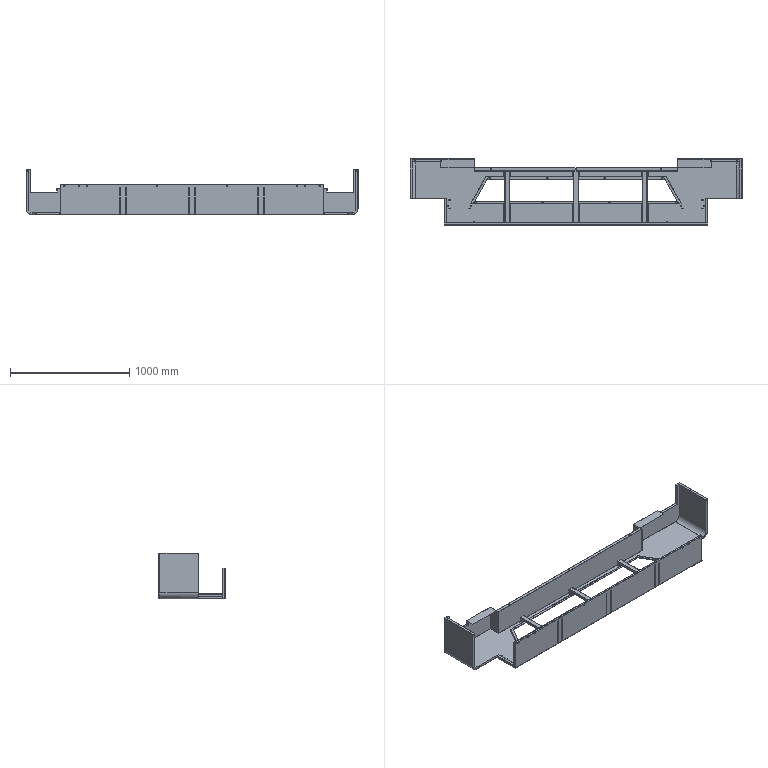Part | SolidWorks | features ReferencePattern 7, MirrorCompFeat 2, LocalLPattern 1 | 16 solids | 918 faces | box 2780 x 555 x 380 mm | volume 4361230 mm3 | plane 657 | cylinder 229 | spline 32 | commonest cylinder face diameters 6 x74 1 x32 4 x32 2 x30 5 x30 10 x16